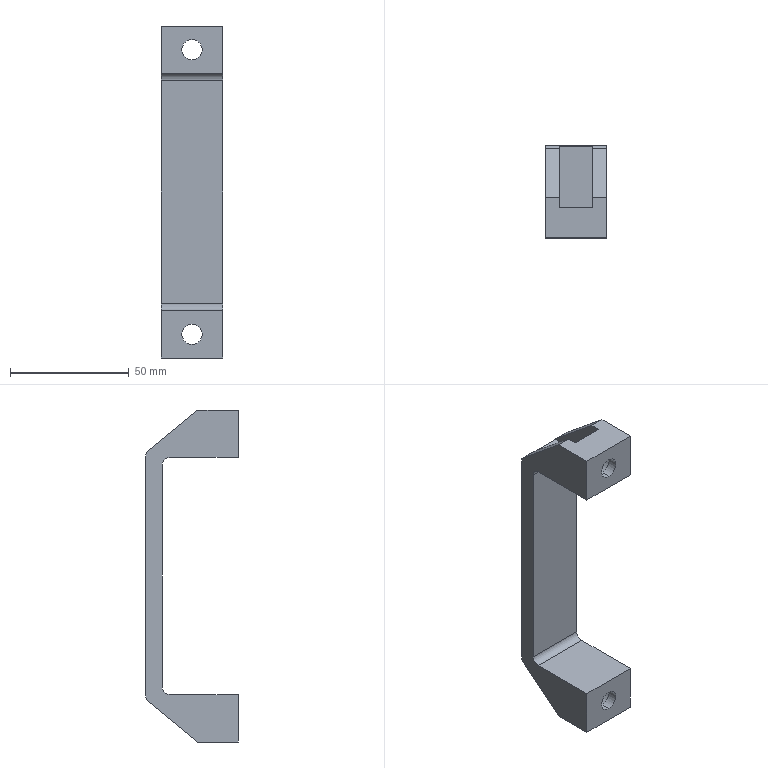Part | SolidWorks | features BaseBody 1 | 1 solid | 38 faces | box 26 x 39 x 140 mm | volume 37768 mm3 | plane 26 | cylinder 12 | commonest cylinder face diameters 6 x4 8.5 x4 14 x4
STEP:
#1=CARTESIAN_POINT('',(0.,-39.,-55.75));
#2=VERTEX_POINT('',#1);
#3=CARTESIAN_POINT('',(0.,-39.,-64.25));
#4=VERTEX_POINT('',#3);
#5=CARTESIAN_POINT('',(0.,-39.,-60.));
#6=DIRECTION('',(0.,-1.,0.));
#7=DIRECTION('',(0.,0.,1.));
#8=AXIS2_PLACEMENT_3D('',#5,#6,#7);
#9=CIRCLE('',#8,4.25);
#10=EDGE_CURVE('',#2,#4,#9,.T.);
#11=ORIENTED_EDGE('',*,*,#10,.T.);
#12=CARTESIAN_POINT('',(0.,-35.,-64.25));
#13=VERTEX_POINT('',#12);
#14=CARTESIAN_POINT('',(0.,-50.,-64.25));
#15=DIRECTION('',(0.,1.,0.));
#16=VECTOR('',#15,1000.);
#17=LINE('',#14,#16);
#18=EDGE_CURVE('',#4,#13,#17,.T.);
#19=ORIENTED_EDGE('',*,*,#18,.T.);
#20=CARTESIAN_POINT('',(0.,-35.,-55.75));
#21=VERTEX_POINT('',#20);
#22=CARTESIAN_POINT('',(0.,-35.,-60.));
#23=DIRECTION('',(0.,-1.,0.));
#24=DIRECTION('',(0.,0.,1.));
#25=AXIS2_PLACEMENT_3D('',#22,#23,#24);
#26=CIRCLE('',#25,4.25);
#27=EDGE_CURVE('',#21,#13,#26,.T.);
#28=ORIENTED_EDGE('',*,*,#27,.F.);
#29=CARTESIAN_POINT('',(0.,-50.,-55.75));
#30=DIRECTION('',(0.,1.,0.));
#31=VECTOR('',#30,1000.);
#32=LINE('',#29,#31);
#33=EDGE_CURVE('',#2,#21,#32,.T.);
#34=ORIENTED_EDGE('',*,*,#33,.F.);
#35=EDGE_LOOP('',(#11,#19,#28,#34));
#36=FACE_OUTER_BOUND('',#35,.T.);
#37=CARTESIAN_POINT('',(0.,-50.,-60.));
#38=DIRECTION('',(0.,1.,0.));
#39=DIRECTION('',(0.,0.,1.));
#40=AXIS2_PLACEMENT_3D('',#37,#38,#39);
#41=CYLINDRICAL_SURFACE('',#40,4.25);
#42=ADVANCED_FACE('',(#36),#41,.F.);
#43=CARTESIAN_POINT('',(0.,-35.,64.25));
#44=VERTEX_POINT('',#43);
#45=CARTESIAN_POINT('',(0.,-35.,55.75));
#46=VERTEX_POINT('',#45);
#47=CARTESIAN_POINT('',(0.,-35.,60.));
#48=DIRECTION('',(0.,-1.,0.));
#49=DIRECTION('',(0.,0.,-1.));
#50=AXIS2_PLACEMENT_3D('',#47,#48,#49);
#51=CIRCLE('',#50,4.25);
#52=EDGE_CURVE('',#44,#46,#51,.T.);
#53=ORIENTED_EDGE('',*,*,#52,.F.);
#54=CARTESIAN_POINT('',(0.,-39.,64.25));
#55=VERTEX_POINT('',#54);
#56=CARTESIAN_POINT('',(0.,50.,64.25));
#57=DIRECTION('',(0.,-1.,0.));
#58=VECTOR('',#57,1000.);
#59=LINE('',#56,#58);
#60=EDGE_CURVE('',#44,#55,#59,.T.);
#61=ORIENTED_EDGE('',*,*,#60,.T.);
#62=CARTESIAN_POINT('',(0.,-39.,55.75));
#63=VERTEX_POINT('',#62);
#64=CARTESIAN_POINT('',(0.,-39.,60.));
#65=DIRECTION('',(0.,-1.,0.));
#66=DIRECTION('',(0.,0.,-1.));
#67=AXIS2_PLACEMENT_3D('',#64,#65,#66);
#68=CIRCLE('',#67,4.25);
#69=EDGE_CURVE('',#55,#63,#68,.T.);
#70=ORIENTED_EDGE('',*,*,#69,.T.);
#71=CARTESIAN_POINT('',(0.,50.,55.75));
#72=DIRECTION('',(0.,-1.,0.));
#73=VECTOR('',#72,1000.);
#74=LINE('',#71,#73);
#75=EDGE_CURVE('',#46,#63,#74,.T.);
#76=ORIENTED_EDGE('',*,*,#75,.F.);
#77=EDGE_LOOP('',(#53,#61,#70,#76));
#78=FACE_OUTER_BOUND('',#77,.T.);
#79=CARTESIAN_POINT('',(0.,50.,60.));
#80=DIRECTION('',(0.,-1.,0.));
#81=DIRECTION('',(0.,0.,-1.));
#82=AXIS2_PLACEMENT_3D('',#79,#80,#81);
#83=CYLINDRICAL_SURFACE('',#82,4.25);
#84=ADVANCED_FACE('',(#78),#83,.F.);
#85=CARTESIAN_POINT('',(0.,-35.,-67.));
#86=VERTEX_POINT('',#85);
#87=CARTESIAN_POINT('',(0.,-35.,-53.));
#88=VERTEX_POINT('',#87);
#89=CARTESIAN_POINT('',(0.,-35.,-60.));
#90=DIRECTION('',(0.,1.,0.));
#91=DIRECTION('',(0.,0.,1.));
#92=AXIS2_PLACEMENT_3D('',#89,#90,#91);
#93=CIRCLE('',#92,7.);
#94=EDGE_CURVE('',#86,#88,#93,.T.);
#95=ORIENTED_EDGE('',*,*,#94,.F.);
#96=CARTESIAN_POINT('',(0.,-26.,-67.));
#97=VERTEX_POINT('',#96);
#98=CARTESIAN_POINT('',(0.,-50.,-67.));
#99=DIRECTION('',(0.,1.,0.));
#100=VECTOR('',#99,1000.);
#101=LINE('',#98,#100);
#102=EDGE_CURVE('',#86,#97,#101,.T.);
#103=ORIENTED_EDGE('',*,*,#102,.T.);
#104=CARTESIAN_POINT('',(-7.,-26.,-60.));
#105=VERTEX_POINT('',#104);
#106=CARTESIAN_POINT('',(0.,-26.,-60.));
#107=DIRECTION('',(0.,-1.,0.));
#108=DIRECTION('',(0.,0.,1.));
#109=AXIS2_PLACEMENT_3D('',#106,#107,#108);
#110=CIRCLE('',#109,7.);
#111=EDGE_CURVE('',#105,#97,#110,.T.);
#112=ORIENTED_EDGE('',*,*,#111,.F.);
#113=CARTESIAN_POINT('',(0.,-26.,-53.));
#114=VERTEX_POINT('',#113);
#115=CARTESIAN_POINT('',(0.,-26.,-60.));
#116=DIRECTION('',(0.,-1.,0.));
#117=DIRECTION('',(0.,0.,1.));
#118=AXIS2_PLACEMENT_3D('',#115,#116,#117);
#119=CIRCLE('',#118,7.);
#120=EDGE_CURVE('',#114,#105,#119,.T.);
#121=ORIENTED_EDGE('',*,*,#120,.F.);
#122=CARTESIAN_POINT('',(0.,-50.,-53.));
#123=DIRECTION('',(0.,1.,0.));
#124=VECTOR('',#123,1000.);
#125=LINE('',#122,#124);
#126=EDGE_CURVE('',#88,#114,#125,.T.);
#127=ORIENTED_EDGE('',*,*,#126,.F.);
#128=EDGE_LOOP('',(#95,#103,#112,#121,#127));
#129=FACE_OUTER_BOUND('',#128,.T.);
#130=CARTESIAN_POINT('',(0.,-50.,-60.));
#131=DIRECTION('',(0.,1.,0.));
#132=DIRECTION('',(0.,0.,1.));
#133=AXIS2_PLACEMENT_3D('',#130,#131,#132);
#134=CYLINDRICAL_SURFACE('',#133,7.);
#135=ADVANCED_FACE('',(#129),#134,.F.);
#136=CARTESIAN_POINT('',(0.,-26.,67.));
#137=VERTEX_POINT('',#136);
#138=CARTESIAN_POINT('',(-7.,-26.,60.));
#139=VERTEX_POINT('',#138);
#140=CARTESIAN_POINT('',(0.,-26.,60.));
#141=DIRECTION('',(0.,-1.,0.));
#142=DIRECTION('',(0.,0.,-1.));
#143=AXIS2_PLACEMENT_3D('',#140,#141,#142);
#144=CIRCLE('',#143,7.);
#145=EDGE_CURVE('',#137,#139,#144,.T.);
#146=ORIENTED_EDGE('',*,*,#145,.F.);
#147=CARTESIAN_POINT('',(0.,-35.,67.));
#148=VERTEX_POINT('',#147);
#149=CARTESIAN_POINT('',(0.,50.,67.));
#150=DIRECTION('',(0.,-1.,0.));
#151=VECTOR('',#150,1000.);
#152=LINE('',#149,#151);
#153=EDGE_CURVE('',#137,#148,#152,.T.);
#154=ORIENTED_EDGE('',*,*,#153,.T.);
#155=CARTESIAN_POINT('',(0.,-35.,53.));
#156=VERTEX_POINT('',#155);
#157=CARTESIAN_POINT('',(0.,-35.,60.));
#158=DIRECTION('',(0.,1.,0.));
#159=DIRECTION('',(0.,0.,-1.));
#160=AXIS2_PLACEMENT_3D('',#157,#158,#159);
#161=CIRCLE('',#160,7.);
#162=EDGE_CURVE('',#156,#148,#161,.T.);
#163=ORIENTED_EDGE('',*,*,#162,.F.);
#164=CARTESIAN_POINT('',(0.,-26.,53.));
#165=VERTEX_POINT('',#164);
#166=CARTESIAN_POINT('',(0.,50.,53.));
#167=DIRECTION('',(0.,-1.,0.));
#168=VECTOR('',#167,1000.);
#169=LINE('',#166,#168);
#170=EDGE_CURVE('',#165,#156,#169,.T.);
#171=ORIENTED_EDGE('',*,*,#170,.F.);
#172=CARTESIAN_POINT('',(0.,-26.,60.));
#173=DIRECTION('',(0.,-1.,0.));
#174=DIRECTION('',(0.,0.,-1.));
#175=AXIS2_PLACEMENT_3D('',#172,#173,#174);
#176=CIRCLE('',#175,7.);
#177=EDGE_CURVE('',#139,#165,#176,.T.);
#178=ORIENTED_EDGE('',*,*,#177,.F.);
#179=EDGE_LOOP('',(#146,#154,#163,#171,#178));
#180=FACE_OUTER_BOUND('',#179,.T.);
#181=CARTESIAN_POINT('',(0.,50.,60.));
#182=DIRECTION('',(0.,-1.,0.));
#183=DIRECTION('',(0.,0.,-1.));
#184=AXIS2_PLACEMENT_3D('',#181,#182,#183);
#185=CYLINDRICAL_SURFACE('',#184,7.);
#186=ADVANCED_FACE('',(#180),#185,.F.);
#187=CARTESIAN_POINT('',(13.,0.,50.578));
#188=VERTEX_POINT('',#187);
#189=CARTESIAN_POINT('',(-13.,0.,50.578));
#190=VERTEX_POINT('',#189);
#191=CARTESIAN_POINT('',(13.,0.,50.578));
#192=DIRECTION('',(-1.,0.,0.));
#193=VECTOR('',#192,1000.);
#194=LINE('',#191,#193);
#195=EDGE_CURVE('',#188,#190,#194,.T.);
#196=ORIENTED_EDGE('',*,*,#195,.F.);
#197=CARTESIAN_POINT('',(13.,0.,-50.578));
#198=VERTEX_POINT('',#197);
#199=CARTESIAN_POINT('',(13.,0.,-50.578));
#200=DIRECTION('',(0.,0.,1.));
#201=VECTOR('',#200,1000.);
#202=LINE('',#199,#201);
#203=EDGE_CURVE('',#198,#188,#202,.T.);
#204=ORIENTED_EDGE('',*,*,#203,.F.);
#205=CARTESIAN_POINT('',(-13.,0.,-50.578));
#206=VERTEX_POINT('',#205);
#207=CARTESIAN_POINT('',(13.,0.,-50.578));
#208=DIRECTION('',(1.,0.,0.));
#209=VECTOR('',#208,1000.);
#210=LINE('',#207,#209);
#211=EDGE_CURVE('',#206,#198,#210,.T.);
#212=ORIENTED_EDGE('',*,*,#211,.F.);
#213=CARTESIAN_POINT('',(-13.,0.,-50.578));
#214=DIRECTION('',(0.,0.,-1.));
#215=VECTOR('',#214,1000.);
#216=LINE('',#213,#215);
#217=EDGE_CURVE('',#190,#206,#216,.T.);
#218=ORIENTED_EDGE('',*,*,#217,.F.);
#219=EDGE_LOOP('',(#196,#204,#212,#218));
#220=FACE_OUTER_BOUND('',#219,.T.);
#221=CARTESIAN_POINT('',(13.,0.,-50.578));
#222=DIRECTION('',(0.,-1.,0.));
#223=DIRECTION('',(0.,0.,-1.));
#224=AXIS2_PLACEMENT_3D('',#221,#222,#223);
#225=PLANE('',#224);
#226=ADVANCED_FACE('',(#220),#225,.F.);
#227=ORIENTED_EDGE('',*,*,#217,.T.);
#228=CARTESIAN_POINT('',(-13.,-1.1,-52.9));
#229=VERTEX_POINT('',#228);
#230=CARTESIAN_POINT('',(-13.,-3.,-50.578));
#231=DIRECTION('',(1.,0.,0.));
#232=DIRECTION('',(0.,0.,-1.));
#233=AXIS2_PLACEMENT_3D('',#230,#231,#232);
#234=CIRCLE('',#233,3.);
#235=EDGE_CURVE('',#229,#206,#234,.T.);
#236=ORIENTED_EDGE('',*,*,#235,.F.);
#237=CARTESIAN_POINT('',(-13.,-22.,-70.));
#238=VERTEX_POINT('',#237);
#239=CARTESIAN_POINT('',(-13.,-22.,-70.));
#240=DIRECTION('',(0.,0.774,0.6332));
#241=VECTOR('',#240,1000.);
#242=LINE('',#239,#241);
#243=EDGE_CURVE('',#238,#229,#242,.T.);
#244=ORIENTED_EDGE('',*,*,#243,.F.);
#245=CARTESIAN_POINT('',(-13.,-39.,-70.));
#246=VERTEX_POINT('',#245);
#247=CARTESIAN_POINT('',(-13.,-10.,-70.));
#248=DIRECTION('',(0.,1.,0.));
#249=VECTOR('',#248,1000.);
#250=LINE('',#247,#249);
#251=EDGE_CURVE('',#246,#238,#250,.T.);
#252=ORIENTED_EDGE('',*,*,#251,.F.);
#253=CARTESIAN_POINT('',(-13.,-39.,-50.));
#254=VERTEX_POINT('',#253);
#255=CARTESIAN_POINT('',(-13.,-39.,47.));
#256=DIRECTION('',(0.,0.,-1.));
#257=VECTOR('',#256,1000.);
#258=LINE('',#255,#257);
#259=EDGE_CURVE('',#254,#246,#258,.T.);
#260=ORIENTED_EDGE('',*,*,#259,.F.);
#261=CARTESIAN_POINT('',(-13.,-10.,-50.));
#262=VERTEX_POINT('',#261);
#263=CARTESIAN_POINT('',(-13.,-10.,-50.));
#264=DIRECTION('',(0.,-1.,0.));
#265=VECTOR('',#264,1000.);
#266=LINE('',#263,#265);
#267=EDGE_CURVE('',#262,#254,#266,.T.);
#268=ORIENTED_EDGE('',*,*,#267,.F.);
#269=CARTESIAN_POINT('',(-13.,-7.,-47.));
#270=VERTEX_POINT('',#269);
#271=CARTESIAN_POINT('',(-13.,-10.,-47.));
#272=DIRECTION('',(-1.,0.,0.));
#273=DIRECTION('',(0.,0.,-1.));
#274=AXIS2_PLACEMENT_3D('',#271,#272,#273);
#275=CIRCLE('',#274,3.);
#276=EDGE_CURVE('',#270,#262,#275,.T.);
#277=ORIENTED_EDGE('',*,*,#276,.F.);
#278=CARTESIAN_POINT('',(-13.,-7.,47.));
#279=VERTEX_POINT('',#278);
#280=CARTESIAN_POINT('',(-13.,-7.,47.));
#281=DIRECTION('',(0.,0.,-1.));
#282=VECTOR('',#281,1000.);
#283=LINE('',#280,#282);
#284=EDGE_CURVE('',#279,#270,#283,.T.);
#285=ORIENTED_EDGE('',*,*,#284,.F.);
#286=CARTESIAN_POINT('',(-13.,-10.,50.));
#287=VERTEX_POINT('',#286);
#288=CARTESIAN_POINT('',(-13.,-10.,47.));
#289=DIRECTION('',(-1.,0.,0.));
#290=DIRECTION('',(0.,0.,-1.));
#291=AXIS2_PLACEMENT_3D('',#288,#289,#290);
#292=CIRCLE('',#291,3.);
#293=EDGE_CURVE('',#287,#279,#292,.T.);
#294=ORIENTED_EDGE('',*,*,#293,.F.);
#295=CARTESIAN_POINT('',(-13.,-39.,50.));
#296=VERTEX_POINT('',#295);
#297=CARTESIAN_POINT('',(-13.,-10.,50.));
#298=DIRECTION('',(0.,1.,0.));
#299=VECTOR('',#298,1000.);
#300=LINE('',#297,#299);
#301=EDGE_CURVE('',#296,#287,#300,.T.);
#302=ORIENTED_EDGE('',*,*,#301,.F.);
#303=CARTESIAN_POINT('',(-13.,-39.,70.));
#304=VERTEX_POINT('',#303);
#305=CARTESIAN_POINT('',(-13.,-39.,47.));
#306=DIRECTION('',(0.,0.,-1.));
#307=VECTOR('',#306,1000.);
#308=LINE('',#305,#307);
#309=EDGE_CURVE('',#304,#296,#308,.T.);
#310=ORIENTED_EDGE('',*,*,#309,.F.);
#311=CARTESIAN_POINT('',(-13.,-22.,70.));
#312=VERTEX_POINT('',#311);
#313=CARTESIAN_POINT('',(-13.,-10.,70.));
#314=DIRECTION('',(0.,-1.,0.));
#315=VECTOR('',#314,1000.);
#316=LINE('',#313,#315);
#317=EDGE_CURVE('',#312,#304,#316,.T.);
#318=ORIENTED_EDGE('',*,*,#317,.F.);
#319=CARTESIAN_POINT('',(-13.,-1.1,52.9));
#320=VERTEX_POINT('',#319);
#321=CARTESIAN_POINT('',(-13.,-1.1,52.9));
#322=DIRECTION('',(0.,-0.774,0.6332));
#323=VECTOR('',#322,1000.);
#324=LINE('',#321,#323);
#325=EDGE_CURVE('',#320,#312,#324,.T.);
#326=ORIENTED_EDGE('',*,*,#325,.F.);
#327=CARTESIAN_POINT('',(-13.,-3.,50.578));
#328=DIRECTION('',(1.,0.,0.));
#329=DIRECTION('',(0.,0.,-1.));
#330=AXIS2_PLACEMENT_3D('',#327,#328,#329);
#331=CIRCLE('',#330,3.);
#332=EDGE_CURVE('',#190,#320,#331,.T.);
#333=ORIENTED_EDGE('',*,*,#332,.F.);
#334=EDGE_LOOP('',(#227,#236,#244,#252,#260,#268,#277,#285,#294,#302,#310,#318,#326,#333));
#335=FACE_OUTER_BOUND('',#334,.T.);
#336=CARTESIAN_POINT('',(-13.,-10.,47.));
#337=DIRECTION('',(1.,0.,0.));
#338=DIRECTION('',(0.,0.,-1.));
#339=AXIS2_PLACEMENT_3D('',#336,#337,#338);
#340=PLANE('',#339);
#341=ADVANCED_FACE('',(#335),#340,.F.);
#342=ORIENTED_EDGE('',*,*,#195,.T.);
#343=ORIENTED_EDGE('',*,*,#332,.T.);
#344=CARTESIAN_POINT('',(-7.,-1.1,52.9));
#345=VERTEX_POINT('',#344);
#346=CARTESIAN_POINT('',(13.,-1.1,52.9));
#347=DIRECTION('',(1.,0.,0.));
#348=VECTOR('',#347,1000.);
#349=LINE('',#346,#348);
#350=EDGE_CURVE('',#320,#345,#349,.T.);
#351=ORIENTED_EDGE('',*,*,#350,.T.);
#352=CARTESIAN_POINT('',(-7.,-0.3582,52.));
#353=VERTEX_POINT('',#352);
#354=CARTESIAN_POINT('',(-7.,-3.,50.578));
#355=DIRECTION('',(1.,0.,0.));
#356=DIRECTION('',(0.,0.,-1.));
#357=AXIS2_PLACEMENT_3D('',#354,#355,#356);
#358=CIRCLE('',#357,3.);
#359=EDGE_CURVE('',#353,#345,#358,.T.);
#360=ORIENTED_EDGE('',*,*,#359,.F.);
#361=CARTESIAN_POINT('',(7.,-0.3582,52.));
#362=VERTEX_POINT('',#361);
#363=CARTESIAN_POINT('',(13.,-0.3582,52.));
#364=DIRECTION('',(1.,0.,0.));
#365=VECTOR('',#364,1000.);
#366=LINE('',#363,#365);
#367=EDGE_CURVE('',#353,#362,#366,.T.);
#368=ORIENTED_EDGE('',*,*,#367,.T.);
#369=CARTESIAN_POINT('',(7.,-1.1,52.9));
#370=VERTEX_POINT('',#369);
#371=CARTESIAN_POINT('',(7.,-3.,50.578));
#372=DIRECTION('',(1.,0.,0.));
#373=DIRECTION('',(0.,0.,-1.));
#374=AXIS2_PLACEMENT_3D('',#371,#372,#373);
#375=CIRCLE('',#374,3.);
#376=EDGE_CURVE('',#362,#370,#375,.T.);
#377=ORIENTED_EDGE('',*,*,#376,.T.);
#378=CARTESIAN_POINT('',(13.,-1.1,52.9));
#379=VERTEX_POINT('',#378);
#380=CARTESIAN_POINT('',(13.,-1.1,52.9));
#381=DIRECTION('',(1.,0.,0.));
#382=VECTOR('',#381,1000.);
#383=LINE('',#380,#382);
#384=EDGE_CURVE('',#370,#379,#383,.T.);
#385=ORIENTED_EDGE('',*,*,#384,.T.);
#386=CARTESIAN_POINT('',(13.,-3.,50.578));
#387=DIRECTION('',(-1.,0.,0.));
#388=DIRECTION('',(0.,0.,-1.));
#389=AXIS2_PLACEMENT_3D('',#386,#387,#388);
#390=CIRCLE('',#389,3.);
#391=EDGE_CURVE('',#379,#188,#390,.T.);
#392=ORIENTED_EDGE('',*,*,#391,.T.);
#393=EDGE_LOOP('',(#342,#343,#351,#360,#368,#377,#385,#392));
#394=FACE_OUTER_BOUND('',#393,.T.);
#395=CARTESIAN_POINT('',(13.,-3.,50.578));
#396=DIRECTION('',(1.,0.,0.));
#397=DIRECTION('',(0.,0.,-1.));
#398=AXIS2_PLACEMENT_3D('',#395,#396,#397);
#399=CYLINDRICAL_SURFACE('',#398,3.);
#400=ADVANCED_FACE('',(#394),#399,.T.);
#401=CARTESIAN_POINT('',(13.,-22.,-70.));
#402=VERTEX_POINT('',#401);
#403=CARTESIAN_POINT('',(13.,-1.1,-52.9));
#404=VERTEX_POINT('',#403);
#405=CARTESIAN_POINT('',(13.,-22.,-70.));
#406=DIRECTION('',(0.,0.774,0.6332));
#407=VECTOR('',#406,1000.);
#408=LINE('',#405,#407);
#409=EDGE_CURVE('',#402,#404,#408,.T.);
#410=ORIENTED_EDGE('',*,*,#409,.T.);
#411=CARTESIAN_POINT('',(13.,-3.,-50.578));
#412=DIRECTION('',(1.,0.,0.));
#413=DIRECTION('',(0.,0.,-1.));
#414=AXIS2_PLACEMENT_3D('',#411,#412,#413);
#415=CIRCLE('',#414,3.);
#416=EDGE_CURVE('',#404,#198,#415,.T.);
#417=ORIENTED_EDGE('',*,*,#416,.T.);
#418=ORIENTED_EDGE('',*,*,#203,.T.);
#419=ORIENTED_EDGE('',*,*,#391,.F.);
#420=CARTESIAN_POINT('',(13.,-22.,70.));
#421=VERTEX_POINT('',#420);
#422=CARTESIAN_POINT('',(13.,-1.1,52.9));
#423=DIRECTION('',(0.,-0.774,0.6332));
#424=VECTOR('',#423,1000.);
#425=LINE('',#422,#424);
#426=EDGE_CURVE('',#379,#421,#425,.T.);
#427=ORIENTED_EDGE('',*,*,#426,.T.);
#428=CARTESIAN_POINT('',(13.,-39.,70.));
#429=VERTEX_POINT('',#428);
#430=CARTESIAN_POINT('',(13.,-10.,70.));
#431=DIRECTION('',(0.,-1.,0.));
#432=VECTOR('',#431,1000.);
#433=LINE('',#430,#432);
#434=EDGE_CURVE('',#421,#429,#433,.T.);
#435=ORIENTED_EDGE('',*,*,#434,.T.);
#436=CARTESIAN_POINT('',(13.,-39.,50.));
#437=VERTEX_POINT('',#436);
#438=CARTESIAN_POINT('',(13.,-39.,47.));
#439=DIRECTION('',(0.,0.,-1.));
#440=VECTOR('',#439,1000.);
#441=LINE('',#438,#440);
#442=EDGE_CURVE('',#429,#437,#441,.T.);
#443=ORIENTED_EDGE('',*,*,#442,.T.);
#444=CARTESIAN_POINT('',(13.,-10.,50.));
#445=VERTEX_POINT('',#444);
#446=CARTESIAN_POINT('',(13.,-10.,50.));
#447=DIRECTION('',(0.,1.,0.));
#448=VECTOR('',#447,1000.);
#449=LINE('',#446,#448);
#450=EDGE_CURVE('',#437,#445,#449,.T.);
#451=ORIENTED_EDGE('',*,*,#450,.T.);
#452=CARTESIAN_POINT('',(13.,-7.,47.));
#453=VERTEX_POINT('',#452);
#454=CARTESIAN_POINT('',(13.,-10.,47.));
#455=DIRECTION('',(-1.,0.,0.));
#456=DIRECTION('',(0.,0.,-1.));
#457=AXIS2_PLACEMENT_3D('',#454,#455,#456);
#458=CIRCLE('',#457,3.);
#459=EDGE_CURVE('',#445,#453,#458,.T.);
#460=ORIENTED_EDGE('',*,*,#459,.T.);
#461=CARTESIAN_POINT('',(13.,-7.,-47.));
#462=VERTEX_POINT('',#461);
#463=CARTESIAN_POINT('',(13.,-7.,47.));
#464=DIRECTION('',(0.,0.,-1.));
#465=VECTOR('',#464,1000.);
#466=LINE('',#463,#465);
#467=EDGE_CURVE('',#453,#462,#466,.T.);
#468=ORIENTED_EDGE('',*,*,#467,.T.);
#469=CARTESIAN_POINT('',(13.,-10.,-50.));
#470=VERTEX_POINT('',#469);
#471=CARTESIAN_POINT('',(13.,-10.,-47.));
#472=DIRECTION('',(-1.,0.,0.));
#473=DIRECTION('',(0.,0.,-1.));
#474=AXIS2_PLACEMENT_3D('',#471,#472,#473);
#475=CIRCLE('',#474,3.);
#476=EDGE_CURVE('',#462,#470,#475,.T.);
#477=ORIENTED_EDGE('',*,*,#476,.T.);
#478=CARTESIAN_POINT('',(13.,-39.,-50.));
#479=VERTEX_POINT('',#478);
#480=CARTESIAN_POINT('',(13.,-10.,-50.));
#481=DIRECTION('',(0.,-1.,0.));
#482=VECTOR('',#481,1000.);
#483=LINE('',#480,#482);
#484=EDGE_CURVE('',#470,#479,#483,.T.);
#485=ORIENTED_EDGE('',*,*,#484,.T.);
#486=CARTESIAN_POINT('',(13.,-39.,-70.));
#487=VERTEX_POINT('',#486);
#488=CARTESIAN_POINT('',(13.,-39.,47.));
#489=DIRECTION('',(0.,0.,-1.));
#490=VECTOR('',#489,1000.);
#491=LINE('',#488,#490);
#492=EDGE_CURVE('',#479,#487,#491,.T.);
#493=ORIENTED_EDGE('',*,*,#492,.T.);
#494=CARTESIAN_POINT('',(13.,-10.,-70.));
#495=DIRECTION('',(0.,1.,0.));
#496=VECTOR('',#495,1000.);
#497=LINE('',#494,#496);
#498=EDGE_CURVE('',#487,#402,#497,.T.);
#499=ORIENTED_EDGE('',*,*,#498,.T.);
#500=EDGE_LOOP('',(#410,#417,#418,#419,#427,#435,#443,#451,#460,#468,#477,#485,#493,#499));
#501=FACE_OUTER_BOUND('',#500,.T.);
#502=CARTESIAN_POINT('',(13.,-10.,47.));
#503=DIRECTION('',(1.,0.,0.));
#504=DIRECTION('',(0.,0.,-1.));
#505=AXIS2_PLACEMENT_3D('',#502,#503,#504);
#506=PLANE('',#505);
#507=ADVANCED_FACE('',(#501),#506,.T.);
#508=CARTESIAN_POINT('',(-7.,-1.1,-52.9));
#509=VERTEX_POINT('',#508);
#510=CARTESIAN_POINT('',(13.,-1.1,-52.9));
#511=DIRECTION('',(-1.,0.,0.));
#512=VECTOR('',#511,1000.);
#513=LINE('',#510,#512);
#514=EDGE_CURVE('',#509,#229,#513,.T.);
#515=ORIENTED_EDGE('',*,*,#514,.T.);
#516=ORIENTED_EDGE('',*,*,#235,.T.);
#517=ORIENTED_EDGE('',*,*,#211,.T.);
#518=ORIENTED_EDGE('',*,*,#416,.F.);
#519=CARTESIAN_POINT('',(7.,-1.1,-52.9));
#520=VERTEX_POINT('',#519);
#521=CARTESIAN_POINT('',(13.,-1.1,-52.9));
#522=DIRECTION('',(-1.,0.,0.));
#523=VECTOR('',#522,1000.);
#524=LINE('',#521,#523);
#525=EDGE_CURVE('',#404,#520,#524,.T.);
#526=ORIENTED_EDGE('',*,*,#525,.T.);
#527=CARTESIAN_POINT('',(7.,-0.3582,-52.));
#528=VERTEX_POINT('',#527);
#529=CARTESIAN_POINT('',(7.,-3.,-50.578));
#530=DIRECTION('',(1.,0.,0.));
#531=DIRECTION('',(0.,0.,-1.));
#532=AXIS2_PLACEMENT_3D('',#529,#530,#531);
#533=CIRCLE('',#532,3.);
#534=EDGE_CURVE('',#520,#528,#533,.T.);
#535=ORIENTED_EDGE('',*,*,#534,.T.);
#536=CARTESIAN_POINT('',(-7.,-0.3582,-52.));
#537=VERTEX_POINT('',#536);
#538=CARTESIAN_POINT('',(13.,-0.3582,-52.));
#539=DIRECTION('',(-1.,0.,0.));
#540=VECTOR('',#539,1000.);
#541=LINE('',#538,#540);
#542=EDGE_CURVE('',#528,#537,#541,.T.);
#543=ORIENTED_EDGE('',*,*,#542,.T.);
#544=CARTESIAN_POINT('',(-7.,-3.,-50.578));
#545=DIRECTION('',(1.,0.,0.));
#546=DIRECTION('',(0.,0.,-1.));
#547=AXIS2_PLACEMENT_3D('',#544,#545,#546);
#548=CIRCLE('',#547,3.);
#549=EDGE_CURVE('',#509,#537,#548,.T.);
#550=ORIENTED_EDGE('',*,*,#549,.F.);
#551=EDGE_LOOP('',(#515,#516,#517,#518,#526,#535,#543,#550));
#552=FACE_OUTER_BOUND('',#551,.T.);
#553=CARTESIAN_POINT('',(13.,-3.,-50.578));
#554=DIRECTION('',(1.,0.,0.));
#555=DIRECTION('',(0.,0.,-1.));
#556=AXIS2_PLACEMENT_3D('',#553,#554,#555);
#557=CYLINDRICAL_SURFACE('',#556,3.);
#558=ADVANCED_FACE('',(#552),#557,.T.);
#559=ORIENTED_EDGE('',*,*,#243,.T.);
#560=ORIENTED_EDGE('',*,*,#514,.F.);
#561=CARTESIAN_POINT('',(-7.,-22.,-70.));
#562=VERTEX_POINT('',#561);
#563=CARTESIAN_POINT('',(-7.,-22.,-70.));
#564=DIRECTION('',(0.,0.774,0.6332));
#565=VECTOR('',#564,1000.);
#566=LINE('',#563,#565);
#567=EDGE_CURVE('',#562,#509,#566,.T.);
#568=ORIENTED_EDGE('',*,*,#567,.F.);
#569=CARTESIAN_POINT('',(13.,-22.,-70.));
#570=DIRECTION('',(1.,0.,0.));
#571=VECTOR('',#570,1000.);
#572=LINE('',#569,#571);
#573=EDGE_CURVE('',#238,#562,#572,.T.);
#574=ORIENTED_EDGE('',*,*,#573,.F.);
#575=EDGE_LOOP('',(#559,#560,#568,#574));
#576=FACE_OUTER_BOUND('',#575,.T.);
#577=CARTESIAN_POINT('',(13.,-22.,-70.));
#578=DIRECTION('',(0.,-0.6332,0.774));
#579=DIRECTION('',(0.,-0.774,-0.6332));
#580=AXIS2_PLACEMENT_3D('',#577,#578,#579);
#581=PLANE('',#580);
#582=ADVANCED_FACE('',(#576),#581,.F.);
#583=CARTESIAN_POINT('',(7.,-22.,-70.));
#584=VERTEX_POINT('',#583);
#585=CARTESIAN_POINT('',(13.,-22.,-70.));
#586=DIRECTION('',(-1.,0.,0.));
#587=VECTOR('',#586,1000.);
#588=LINE('',#585,#587);
#589=EDGE_CURVE('',#402,#584,#588,.T.);
#590=ORIENTED_EDGE('',*,*,#589,.F.);
#591=ORIENTED_EDGE('',*,*,#498,.F.);
#592=CARTESIAN_POINT('',(13.,-39.,-70.));
#593=DIRECTION('',(1.,0.,0.));
#594=VECTOR('',#593,1000.);
#595=LINE('',#592,#594);
#596=EDGE_CURVE('',#246,#487,#595,.T.);
#597=ORIENTED_EDGE('',*,*,#596,.F.);
#598=ORIENTED_EDGE('',*,*,#251,.T.);
#599=ORIENTED_EDGE('',*,*,#573,.T.);
#600=CARTESIAN_POINT('',(-7.,-26.,-70.));
#601=VERTEX_POINT('',#600);
#602=CARTESIAN_POINT('',(-7.,-39.,-70.));
#603=DIRECTION('',(0.,1.,0.));
#604=VECTOR('',#603,1000.);
#605=LINE('',#602,#604);
#606=EDGE_CURVE('',#601,#562,#605,.T.);
#607=ORIENTED_EDGE('',*,*,#606,.F.);
#608=CARTESIAN_POINT('',(7.,-26.,-70.));
#609=VERTEX_POINT('',#608);
#610=CARTESIAN_POINT('',(13.,-26.,-70.));
#611=DIRECTION('',(-1.,0.,0.));
#612=VECTOR('',#611,1000.);
#613=LINE('',#610,#612);
#614=EDGE_CURVE('',#609,#601,#613,.T.);
#615=ORIENTED_EDGE('',*,*,#614,.F.);
#616=CARTESIAN_POINT('',(7.,-39.,-70.));
#617=DIRECTION('',(0.,-1.,0.));
#618=VECTOR('',#617,1000.);
#619=LINE('',#616,#618);
#620=EDGE_CURVE('',#584,#609,#619,.T.);
#621=ORIENTED_EDGE('',*,*,#620,.F.);
#622=EDGE_LOOP('',(#590,#591,#597,#598,#599,#607,#615,#621));
#623=FACE_OUTER_BOUND('',#622,.T.);
#624=CARTESIAN_POINT('',(13.,-39.,-70.));
#625=DIRECTION('',(0.,0.,1.));
#626=DIRECTION('',(1.,0.,0.));
#627=AXIS2_PLACEMENT_3D('',#624,#625,#626);
#628=PLANE('',#627);
#629=ADVANCED_FACE('',(#623),#628,.F.);
#630=ORIENTED_EDGE('',*,*,#10,.F.);
#631=CARTESIAN_POINT('',(0.,-39.,-60.));
#632=DIRECTION('',(0.,-1.,0.));
#633=DIRECTION('',(0.,0.,1.));
#634=AXIS2_PLACEMENT_3D('',#631,#632,#633);
#635=CIRCLE('',#634,4.25);
#636=EDGE_CURVE('',#4,#2,#635,.T.);
#637=ORIENTED_EDGE('',*,*,#636,.F.);
#638=EDGE_LOOP('',(#630,#637));
#639=FACE_BOUND('',#638,.T.);
#640=ORIENTED_EDGE('',*,*,#492,.F.);
#641=CARTESIAN_POINT('',(13.,-39.,-50.));
#642=DIRECTION('',(1.,0.,0.));
#643=VECTOR('',#642,1000.);
#644=LINE('',#641,#643);
#645=EDGE_CURVE('',#254,#479,#644,.T.);
#646=ORIENTED_EDGE('',*,*,#645,.F.);
#647=ORIENTED_EDGE('',*,*,#259,.T.);
#648=ORIENTED_EDGE('',*,*,#596,.T.);
#649=EDGE_LOOP('',(#640,#646,#647,#648));
#650=FACE_OUTER_BOUND('',#649,.T.);
#651=CARTESIAN_POINT('',(13.,-39.,-50.));
#652=DIRECTION('',(0.,1.,0.));
#653=DIRECTION('',(0.,0.,1.));
#654=AXIS2_PLACEMENT_3D('',#651,#652,#653);
#655=PLANE('',#654);
#656=ADVANCED_FACE('',(#639,#650),#655,.F.);
#657=ORIENTED_EDGE('',*,*,#484,.F.);
#658=CARTESIAN_POINT('',(13.,-10.,-50.));
#659=DIRECTION('',(1.,0.,0.));
#660=VECTOR('',#659,1000.);
#661=LINE('',#658,#660);
#662=EDGE_CURVE('',#262,#470,#661,.T.);
#663=ORIENTED_EDGE('',*,*,#662,.F.);
#664=ORIENTED_EDGE('',*,*,#267,.T.);
#665=ORIENTED_EDGE('',*,*,#645,.T.);
#666=EDGE_LOOP('',(#657,#663,#664,#665));
#667=FACE_OUTER_BOUND('',#666,.T.);
#668=CARTESIAN_POINT('',(13.,-10.,-50.));
#669=DIRECTION('',(0.,0.,-1.));
#670=DIRECTION('',(-1.,0.,0.));
#671=AXIS2_PLACEMENT_3D('',#668,#669,#670);
#672=PLANE('',#671);
#673=ADVANCED_FACE('',(#667),#672,.F.);
#674=ORIENTED_EDGE('',*,*,#476,.F.);
#675=CARTESIAN_POINT('',(13.,-7.,-47.));
#676=DIRECTION('',(1.,0.,0.));
#677=VECTOR('',#676,1000.);
#678=LINE('',#675,#677);
#679=EDGE_CURVE('',#270,#462,#678,.T.);
#680=ORIENTED_EDGE('',*,*,#679,.F.);
#681=ORIENTED_EDGE('',*,*,#276,.T.);
#682=ORIENTED_EDGE('',*,*,#662,.T.);
#683=EDGE_LOOP('',(#674,#680,#681,#682));
#684=FACE_OUTER_BOUND('',#683,.T.);
#685=CARTESIAN_POINT('',(13.,-10.,-47.));
#686=DIRECTION('',(1.,0.,0.));
#687=DIRECTION('',(0.,0.,-1.));
#688=AXIS2_PLACEMENT_3D('',#685,#686,#687);
#689=CYLINDRICAL_SURFACE('',#688,3.);
#690=ADVANCED_FACE('',(#684),#689,.F.);
#691=ORIENTED_EDGE('',*,*,#467,.F.);
#692=CARTESIAN_POINT('',(13.,-7.,47.));
#693=DIRECTION('',(1.,0.,0.));
#694=VECTOR('',#693,1000.);
#695=LINE('',#692,#694);
#696=EDGE_CURVE('',#279,#453,#695,.T.);
#697=ORIENTED_EDGE('',*,*,#696,.F.);
#698=ORIENTED_EDGE('',*,*,#284,.T.);
#699=ORIENTED_EDGE('',*,*,#679,.T.);
#700=EDGE_LOOP('',(#691,#697,#698,#699));
#701=FACE_OUTER_BOUND('',#700,.T.);
#702=CARTESIAN_POINT('',(13.,-7.,47.));
#703=DIRECTION('',(0.,1.,0.));
#704=DIRECTION('',(0.,0.,1.));
#705=AXIS2_PLACEMENT_3D('',#702,#703,#704);
#706=PLANE('',#705);
#707=ADVANCED_FACE('',(#701),#706,.F.);
#708=ORIENTED_EDGE('',*,*,#459,.F.);
#709=CARTESIAN_POINT('',(13.,-10.,50.));
#710=DIRECTION('',(1.,0.,0.));
#711=VECTOR('',#710,1000.);
#712=LINE('',#709,#711);
#713=EDGE_CURVE('',#287,#445,#712,.T.);
#714=ORIENTED_EDGE('',*,*,#713,.F.);
#715=ORIENTED_EDGE('',*,*,#293,.T.);
#716=ORIENTED_EDGE('',*,*,#696,.T.);
#717=EDGE_LOOP('',(#708,#714,#715,#716));
#718=FACE_OUTER_BOUND('',#717,.T.);
#719=CARTESIAN_POINT('',(13.,-10.,47.));
#720=DIRECTION('',(1.,0.,0.));
#721=DIRECTION('',(0.,0.,-1.));
#722=AXIS2_PLACEMENT_3D('',#719,#720,#721);
#723=CYLINDRICAL_SURFACE('',#722,3.);
#724=ADVANCED_FACE('',(#718),#723,.F.);
#725=ORIENTED_EDGE('',*,*,#450,.F.);
#726=CARTESIAN_POINT('',(13.,-39.,50.));
#727=DIRECTION('',(1.,0.,0.));
#728=VECTOR('',#727,1000.);
#729=LINE('',#726,#728);
#730=EDGE_CURVE('',#296,#437,#729,.T.);
#731=ORIENTED_EDGE('',*,*,#730,.F.);
#732=ORIENTED_EDGE('',*,*,#301,.T.);
#733=ORIENTED_EDGE('',*,*,#713,.T.);
#734=EDGE_LOOP('',(#725,#731,#732,#733));
#735=FACE_OUTER_BOUND('',#734,.T.);
#736=CARTESIAN_POINT('',(13.,-39.,50.));
#737=DIRECTION('',(0.,0.,1.));
#738=DIRECTION('',(1.,0.,0.));
#739=AXIS2_PLACEMENT_3D('',#736,#737,#738);
#740=PLANE('',#739);
#741=ADVANCED_FACE('',(#735),#740,.F.);
#742=CARTESIAN_POINT('',(0.,-39.,60.));
#743=DIRECTION('',(0.,-1.,0.));
#744=DIRECTION('',(0.,0.,-1.));
#745=AXIS2_PLACEMENT_3D('',#742,#743,#744);
#746=CIRCLE('',#745,4.25);
#747=EDGE_CURVE('',#63,#55,#746,.T.);
#748=ORIENTED_EDGE('',*,*,#747,.F.);
#749=ORIENTED_EDGE('',*,*,#69,.F.);
#750=EDGE_LOOP('',(#748,#749));
#751=FACE_BOUND('',#750,.T.);
#752=ORIENTED_EDGE('',*,*,#442,.F.);
#753=CARTESIAN_POINT('',(13.,-39.,70.));
#754=DIRECTION('',(1.,0.,0.));
#755=VECTOR('',#754,1000.);
#756=LINE('',#753,#755);
#757=EDGE_CURVE('',#304,#429,#756,.T.);
#758=ORIENTED_EDGE('',*,*,#757,.F.);
#759=ORIENTED_EDGE('',*,*,#309,.T.);
#760=ORIENTED_EDGE('',*,*,#730,.T.);
#761=EDGE_LOOP('',(#752,#758,#759,#760));
#762=FACE_OUTER_BOUND('',#761,.T.);
#763=CARTESIAN_POINT('',(13.,-39.,70.));
#764=DIRECTION('',(0.,1.,0.));
#765=DIRECTION('',(0.,0.,1.));
#766=AXIS2_PLACEMENT_3D('',#763,#764,#765);
#767=PLANE('',#766);
#768=ADVANCED_FACE('',(#751,#762),#767,.F.);
#769=CARTESIAN_POINT('',(-7.,-26.,70.));
#770=VERTEX_POINT('',#769);
#771=CARTESIAN_POINT('',(7.,-26.,70.));
#772=VERTEX_POINT('',#771);
#773=CARTESIAN_POINT('',(13.,-26.,70.));
#774=DIRECTION('',(1.,0.,0.));
#775=VECTOR('',#774,1000.);
#776=LINE('',#773,#775);
#777=EDGE_CURVE('',#770,#772,#776,.T.);
#778=ORIENTED_EDGE('',*,*,#777,.F.);
#779=CARTESIAN_POINT('',(-7.,-22.,70.));
#780=VERTEX_POINT('',#779);
#781=CARTESIAN_POINT('',(-7.,-22.,70.));
#782=DIRECTION('',(0.,-1.,0.));
#783=VECTOR('',#782,1000.);
#784=LINE('',#781,#783);
#785=EDGE_CURVE('',#780,#770,#784,.T.);
#786=ORIENTED_EDGE('',*,*,#785,.F.);
#787=CARTESIAN_POINT('',(13.,-22.,70.));
#788=DIRECTION('',(1.,0.,0.));
#789=VECTOR('',#788,1000.);
#790=LINE('',#787,#789);
#791=EDGE_CURVE('',#312,#780,#790,.T.);
#792=ORIENTED_EDGE('',*,*,#791,.F.);
#793=ORIENTED_EDGE('',*,*,#317,.T.);
#794=ORIENTED_EDGE('',*,*,#757,.T.);
#795=ORIENTED_EDGE('',*,*,#434,.F.);
#796=CARTESIAN_POINT('',(7.,-22.,70.));
#797=VERTEX_POINT('',#796);
#798=CARTESIAN_POINT('',(13.,-22.,70.));
#799=DIRECTION('',(1.,0.,0.));
#800=VECTOR('',#799,1000.);
#801=LINE('',#798,#800);
#802=EDGE_CURVE('',#797,#421,#801,.T.);
#803=ORIENTED_EDGE('',*,*,#802,.F.);
#804=CARTESIAN_POINT('',(7.,-22.,70.));
#805=DIRECTION('',(0.,1.,0.));
#806=VECTOR('',#805,1000.);
#807=LINE('',#804,#806);
#808=EDGE_CURVE('',#772,#797,#807,.T.);
#809=ORIENTED_EDGE('',*,*,#808,.F.);
#810=EDGE_LOOP('',(#778,#786,#792,#793,#794,#795,#803,#809));
#811=FACE_OUTER_BOUND('',#810,.T.);
#812=CARTESIAN_POINT('',(13.,-22.,70.));
#813=DIRECTION('',(0.,0.,-1.));
#814=DIRECTION('',(-1.,0.,0.));
#815=AXIS2_PLACEMENT_3D('',#812,#813,#814);
#816=PLANE('',#815);
#817=ADVANCED_FACE('',(#811),#816,.F.);
#818=ORIENTED_EDGE('',*,*,#325,.T.);
#819=ORIENTED_EDGE('',*,*,#791,.T.);
#820=CARTESIAN_POINT('',(-7.,-1.1,52.9));
#821=DIRECTION('',(0.,-0.774,0.6332));
#822=VECTOR('',#821,1000.);
#823=LINE('',#820,#822);
#824=EDGE_CURVE('',#345,#780,#823,.T.);
#825=ORIENTED_EDGE('',*,*,#824,.F.);
#826=ORIENTED_EDGE('',*,*,#350,.F.);
#827=EDGE_LOOP('',(#818,#819,#825,#826));
#828=FACE_OUTER_BOUND('',#827,.T.);
#829=CARTESIAN_POINT('',(13.,-1.1,52.9));
#830=DIRECTION('',(0.,-0.6332,-0.774));
#831=DIRECTION('',(0.,0.774,-0.6332));
#832=AXIS2_PLACEMENT_3D('',#829,#830,#831);
#833=PLANE('',#832);
#834=ADVANCED_FACE('',(#828),#833,.F.);
#835=ORIENTED_EDGE('',*,*,#802,.T.);
#836=ORIENTED_EDGE('',*,*,#426,.F.);
#837=ORIENTED_EDGE('',*,*,#384,.F.);
#838=CARTESIAN_POINT('',(7.,-1.1,52.9));
#839=DIRECTION('',(0.,0.774,-0.6332));
#840=VECTOR('',#839,1000.);
#841=LINE('',#838,#840);
#842=EDGE_CURVE('',#797,#370,#841,.T.);
#843=ORIENTED_EDGE('',*,*,#842,.F.);
#844=EDGE_LOOP('',(#835,#836,#837,#843));
#845=FACE_OUTER_BOUND('',#844,.T.);
#846=CARTESIAN_POINT('',(13.,-1.1,52.9));
#847=DIRECTION('',(0.,-0.6332,-0.774));
#848=DIRECTION('',(0.,0.774,-0.6332));
#849=AXIS2_PLACEMENT_3D('',#846,#847,#848);
#850=PLANE('',#849);
#851=ADVANCED_FACE('',(#845),#850,.F.);
#852=ORIENTED_EDGE('',*,*,#367,.F.);
#853=CARTESIAN_POINT('',(-7.,-26.,52.));
#854=VERTEX_POINT('',#853);
#855=CARTESIAN_POINT('',(-7.,-26.,52.));
#856=DIRECTION('',(0.,-1.,0.));
#857=VECTOR('',#856,1000.);
#858=LINE('',#855,#857);
#859=EDGE_CURVE('',#353,#854,#858,.T.);
#860=ORIENTED_EDGE('',*,*,#859,.T.);
#861=CARTESIAN_POINT('',(7.,-26.,52.));
#862=VERTEX_POINT('',#861);
#863=CARTESIAN_POINT('',(7.,-26.,52.));
#864=DIRECTION('',(1.,0.,0.));
#865=VECTOR('',#864,1000.);
#866=LINE('',#863,#865);
#867=EDGE_CURVE('',#854,#862,#866,.T.);
#868=ORIENTED_EDGE('',*,*,#867,.T.);
#869=CARTESIAN_POINT('',(7.,-26.,52.));
#870=DIRECTION('',(0.,1.,0.));
#871=VECTOR('',#870,1000.);
#872=LINE('',#869,#871);
#873=EDGE_CURVE('',#862,#362,#872,.T.);
#874=ORIENTED_EDGE('',*,*,#873,.T.);
#875=EDGE_LOOP('',(#852,#860,#868,#874));
#876=FACE_OUTER_BOUND('',#875,.T.);
#877=CARTESIAN_POINT('',(7.,-26.,52.));
#878=DIRECTION('',(0.,0.,1.));
#879=DIRECTION('',(1.,0.,0.));
#880=AXIS2_PLACEMENT_3D('',#877,#878,#879);
#881=PLANE('',#880);
#882=ADVANCED_FACE('',(#876),#881,.T.);
#883=ORIENTED_EDGE('',*,*,#525,.F.);
#884=ORIENTED_EDGE('',*,*,#409,.F.);
#885=ORIENTED_EDGE('',*,*,#589,.T.);
#886=CARTESIAN_POINT('',(7.,-22.,-70.));
#887=DIRECTION('',(0.,-0.774,-0.6332));
#888=VECTOR('',#887,1000.);
#889=LINE('',#886,#888);
#890=EDGE_CURVE('',#520,#584,#889,.T.);
#891=ORIENTED_EDGE('',*,*,#890,.F.);
#892=EDGE_LOOP('',(#883,#884,#885,#891));
#893=FACE_OUTER_BOUND('',#892,.T.);
#894=CARTESIAN_POINT('',(13.,-22.,-70.));
#895=DIRECTION('',(0.,-0.6332,0.774));
#896=DIRECTION('',(0.,-0.774,-0.6332));
#897=AXIS2_PLACEMENT_3D('',#894,#895,#896);
#898=PLANE('',#897);
#899=ADVANCED_FACE('',(#893),#898,.F.);
#900=ORIENTED_EDGE('',*,*,#542,.F.);
#901=CARTESIAN_POINT('',(7.,-26.,-52.));
#902=VERTEX_POINT('',#901);
#903=CARTESIAN_POINT('',(7.,0.,-52.));
#904=DIRECTION('',(0.,-1.,0.));
#905=VECTOR('',#904,1000.);
#906=LINE('',#903,#905);
#907=EDGE_CURVE('',#528,#902,#906,.T.);
#908=ORIENTED_EDGE('',*,*,#907,.T.);
#909=CARTESIAN_POINT('',(-7.,-26.,-52.));
#910=VERTEX_POINT('',#909);
#911=CARTESIAN_POINT('',(7.,-26.,-52.));
#912=DIRECTION('',(-1.,0.,0.));
#913=VECTOR('',#912,1000.);
#914=LINE('',#911,#913);
#915=EDGE_CURVE('',#902,#910,#914,.T.);
#916=ORIENTED_EDGE('',*,*,#915,.T.);
#917=CARTESIAN_POINT('',(-7.,0.,-52.));
#918=DIRECTION('',(0.,1.,0.));
#919=VECTOR('',#918,1000.);
#920=LINE('',#917,#919);
#921=EDGE_CURVE('',#910,#537,#920,.T.);
#922=ORIENTED_EDGE('',*,*,#921,.T.);
#923=EDGE_LOOP('',(#900,#908,#916,#922));
#924=FACE_OUTER_BOUND('',#923,.T.);
#925=CARTESIAN_POINT('',(7.,0.,-52.));
#926=DIRECTION('',(0.,0.,-1.));
#927=DIRECTION('',(-1.,0.,0.));
#928=AXIS2_PLACEMENT_3D('',#925,#926,#927);
#929=PLANE('',#928);
#930=ADVANCED_FACE('',(#924),#929,.T.);
#931=ORIENTED_EDGE('',*,*,#921,.F.);
#932=CARTESIAN_POINT('',(-7.,-26.,0.));
#933=DIRECTION('',(0.,0.,-1.));
#934=VECTOR('',#933,1000.);
#935=LINE('',#932,#934);
#936=EDGE_CURVE('',#910,#105,#935,.T.);
#937=ORIENTED_EDGE('',*,*,#936,.T.);
#938=CARTESIAN_POINT('',(-7.,-26.,0.));
#939=DIRECTION('',(0.,0.,-1.));
#940=VECTOR('',#939,1000.);
#941=LINE('',#938,#940);
#942=EDGE_CURVE('',#105,#601,#941,.T.);
#943=ORIENTED_EDGE('',*,*,#942,.T.);
#944=ORIENTED_EDGE('',*,*,#606,.T.);
#945=ORIENTED_EDGE('',*,*,#567,.T.);
#946=ORIENTED_EDGE('',*,*,#549,.T.);
#947=EDGE_LOOP('',(#931,#937,#943,#944,#945,#946));
#948=FACE_OUTER_BOUND('',#947,.T.);
#949=CARTESIAN_POINT('',(-7.,0.,0.));
#950=DIRECTION('',(1.,0.,0.));
#951=DIRECTION('',(0.,0.,-1.));
#952=AXIS2_PLACEMENT_3D('',#949,#950,#951);
#953=PLANE('',#952);
#954=ADVANCED_FACE('',(#948),#953,.T.);
#955=CARTESIAN_POINT('',(7.,-26.,-60.));
#956=VERTEX_POINT('',#955);
#957=CARTESIAN_POINT('',(7.,-26.,0.));
#958=DIRECTION('',(0.,0.,-1.));
#959=VECTOR('',#958,1000.);
#960=LINE('',#957,#959);
#961=EDGE_CURVE('',#902,#956,#960,.T.);
#962=ORIENTED_EDGE('',*,*,#961,.F.);
#963=ORIENTED_EDGE('',*,*,#907,.F.);
#964=ORIENTED_EDGE('',*,*,#534,.F.);
#965=ORIENTED_EDGE('',*,*,#890,.T.);
#966=ORIENTED_EDGE('',*,*,#620,.T.);
#967=CARTESIAN_POINT('',(7.,-26.,0.));
#968=DIRECTION('',(0.,0.,-1.));
#969=VECTOR('',#968,1000.);
#970=LINE('',#967,#969);
#971=EDGE_CURVE('',#956,#609,#970,.T.);
#972=ORIENTED_EDGE('',*,*,#971,.F.);
#973=EDGE_LOOP('',(#962,#963,#964,#965,#966,#972));
#974=FACE_OUTER_BOUND('',#973,.T.);
#975=CARTESIAN_POINT('',(7.,0.,0.));
#976=DIRECTION('',(1.,0.,0.));
#977=DIRECTION('',(0.,0.,-1.));
#978=AXIS2_PLACEMENT_3D('',#975,#976,#977);
#979=PLANE('',#978);
#980=ADVANCED_FACE('',(#974),#979,.F.);
#981=ORIENTED_EDGE('',*,*,#111,.T.);
#982=CARTESIAN_POINT('',(0.,-26.,-60.));
#983=DIRECTION('',(0.,-1.,0.));
#984=DIRECTION('',(0.,0.,1.));
#985=AXIS2_PLACEMENT_3D('',#982,#983,#984);
#986=CIRCLE('',#985,7.);
#987=EDGE_CURVE('',#97,#956,#986,.T.);
#988=ORIENTED_EDGE('',*,*,#987,.T.);
#989=ORIENTED_EDGE('',*,*,#971,.T.);
#990=ORIENTED_EDGE('',*,*,#614,.T.);
#991=ORIENTED_EDGE('',*,*,#942,.F.);
#992=EDGE_LOOP('',(#981,#988,#989,#990,#991));
#993=FACE_OUTER_BOUND('',#992,.T.);
#994=CARTESIAN_POINT('',(7.,-26.,-52.));
#995=DIRECTION('',(0.,1.,0.));
#996=DIRECTION('',(0.,0.,1.));
#997=AXIS2_PLACEMENT_3D('',#994,#995,#996);
#998=PLANE('',#997);
#999=ADVANCED_FACE('',(#993),#998,.T.);
#1000=ORIENTED_EDGE('',*,*,#18,.F.);
#1001=ORIENTED_EDGE('',*,*,#636,.T.);
#1002=ORIENTED_EDGE('',*,*,#33,.T.);
#1003=CARTESIAN_POINT('',(0.,-35.,-60.));
#1004=DIRECTION('',(0.,-1.,0.));
#1005=DIRECTION('',(0.,0.,1.));
#1006=AXIS2_PLACEMENT_3D('',#1003,#1004,#1005);
#1007=CIRCLE('',#1006,4.25);
#1008=EDGE_CURVE('',#13,#21,#1007,.T.);
#1009=ORIENTED_EDGE('',*,*,#1008,.F.);
#1010=EDGE_LOOP('',(#1000,#1001,#1002,#1009));
#1011=FACE_OUTER_BOUND('',#1010,.T.);
#1012=CARTESIAN_POINT('',(0.,-50.,-60.));
#1013=DIRECTION('',(0.,1.,0.));
#1014=DIRECTION('',(0.,0.,1.));
#1015=AXIS2_PLACEMENT_3D('',#1012,#1013,#1014);
#1016=CYLINDRICAL_SURFACE('',#1015,4.25);
#1017=ADVANCED_FACE('',(#1011),#1016,.F.);
#1018=ORIENTED_EDGE('',*,*,#60,.F.);
#1019=CARTESIAN_POINT('',(0.,-35.,60.));
#1020=DIRECTION('',(0.,-1.,0.));
#1021=DIRECTION('',(0.,0.,-1.));
#1022=AXIS2_PLACEMENT_3D('',#1019,#1020,#1021);
#1023=CIRCLE('',#1022,4.25);
#1024=EDGE_CURVE('',#46,#44,#1023,.T.);
#1025=ORIENTED_EDGE('',*,*,#1024,.F.);
#1026=ORIENTED_EDGE('',*,*,#75,.T.);
#1027=ORIENTED_EDGE('',*,*,#747,.T.);
#1028=EDGE_LOOP('',(#1018,#1025,#1026,#1027));
#1029=FACE_OUTER_BOUND('',#1028,.T.);
#1030=CARTESIAN_POINT('',(0.,50.,60.));
#1031=DIRECTION('',(0.,-1.,0.));
#1032=DIRECTION('',(0.,0.,-1.));
#1033=AXIS2_PLACEMENT_3D('',#1030,#1031,#1032);
#1034=CYLINDRICAL_SURFACE('',#1033,4.25);
#1035=ADVANCED_FACE('',(#1029),#1034,.F.);
#1036=CARTESIAN_POINT('',(7.,-26.,60.));
#1037=VERTEX_POINT('',#1036);
#1038=CARTESIAN_POINT('',(7.,-26.,0.));
#1039=DIRECTION('',(0.,0.,-1.));
#1040=VECTOR('',#1039,1000.);
#1041=LINE('',#1038,#1040);
#1042=EDGE_CURVE('',#1037,#862,#1041,.T.);
#1043=ORIENTED_EDGE('',*,*,#1042,.F.);
#1044=CARTESIAN_POINT('',(7.,-26.,0.));
#1045=DIRECTION('',(0.,0.,-1.));
#1046=VECTOR('',#1045,1000.);
#1047=LINE('',#1044,#1046);
#1048=EDGE_CURVE('',#772,#1037,#1047,.T.);
#1049=ORIENTED_EDGE('',*,*,#1048,.F.);
#1050=ORIENTED_EDGE('',*,*,#808,.T.);
#1051=ORIENTED_EDGE('',*,*,#842,.T.);
#1052=ORIENTED_EDGE('',*,*,#376,.F.);
#1053=ORIENTED_EDGE('',*,*,#873,.F.);
#1054=EDGE_LOOP('',(#1043,#1049,#1050,#1051,#1052,#1053));
#1055=FACE_OUTER_BOUND('',#1054,.T.);
#1056=CARTESIAN_POINT('',(7.,0.,0.));
#1057=DIRECTION('',(1.,0.,0.));
#1058=DIRECTION('',(0.,0.,-1.));
#1059=AXIS2_PLACEMENT_3D('',#1056,#1057,#1058);
#1060=PLANE('',#1059);
#1061=ADVANCED_FACE('',(#1055),#1060,.F.);
#1062=ORIENTED_EDGE('',*,*,#1048,.T.);
#1063=CARTESIAN_POINT('',(0.,-26.,60.));
#1064=DIRECTION('',(0.,-1.,0.));
#1065=DIRECTION('',(0.,0.,-1.));
#1066=AXIS2_PLACEMENT_3D('',#1063,#1064,#1065);
#1067=CIRCLE('',#1066,7.);
#1068=EDGE_CURVE('',#1037,#137,#1067,.T.);
#1069=ORIENTED_EDGE('',*,*,#1068,.T.);
#1070=ORIENTED_EDGE('',*,*,#145,.T.);
#1071=CARTESIAN_POINT('',(-7.,-26.,70.));
#1072=DIRECTION('',(0.,0.,1.));
#1073=VECTOR('',#1072,1000.);
#1074=LINE('',#1071,#1073);
#1075=EDGE_CURVE('',#139,#770,#1074,.T.);
#1076=ORIENTED_EDGE('',*,*,#1075,.T.);
#1077=ORIENTED_EDGE('',*,*,#777,.T.);
#1078=EDGE_LOOP('',(#1062,#1069,#1070,#1076,#1077));
#1079=FACE_OUTER_BOUND('',#1078,.T.);
#1080=CARTESIAN_POINT('',(7.,-26.,70.));
#1081=DIRECTION('',(0.,1.,0.));
#1082=DIRECTION('',(0.,0.,1.));
#1083=AXIS2_PLACEMENT_3D('',#1080,#1081,#1082);
#1084=PLANE('',#1083);
#1085=ADVANCED_FACE('',(#1079),#1084,.T.);
#1086=ORIENTED_EDGE('',*,*,#1075,.F.);
#1087=CARTESIAN_POINT('',(-7.,-26.,0.));
#1088=DIRECTION('',(0.,0.,-1.));
#1089=VECTOR('',#1088,1000.);
#1090=LINE('',#1087,#1089);
#1091=EDGE_CURVE('',#139,#854,#1090,.T.);
#1092=ORIENTED_EDGE('',*,*,#1091,.T.);
#1093=ORIENTED_EDGE('',*,*,#859,.F.);
#1094=ORIENTED_EDGE('',*,*,#359,.T.);
#1095=ORIENTED_EDGE('',*,*,#824,.T.);
#1096=ORIENTED_EDGE('',*,*,#785,.T.);
#1097=EDGE_LOOP('',(#1086,#1092,#1093,#1094,#1095,#1096));
#1098=FACE_OUTER_BOUND('',#1097,.T.);
#1099=CARTESIAN_POINT('',(-7.,0.,0.));
#1100=DIRECTION('',(1.,0.,0.));
#1101=DIRECTION('',(0.,0.,-1.));
#1102=AXIS2_PLACEMENT_3D('',#1099,#1100,#1101);
#1103=PLANE('',#1102);
#1104=ADVANCED_FACE('',(#1098),#1103,.T.);
#1105=ORIENTED_EDGE('',*,*,#1091,.F.);
#1106=ORIENTED_EDGE('',*,*,#177,.T.);
#1107=CARTESIAN_POINT('',(0.,-26.,60.));
#1108=DIRECTION('',(0.,-1.,0.));
#1109=DIRECTION('',(0.,0.,-1.));
#1110=AXIS2_PLACEMENT_3D('',#1107,#1108,#1109);
#1111=CIRCLE('',#1110,7.);
#1112=EDGE_CURVE('',#165,#1037,#1111,.T.);
#1113=ORIENTED_EDGE('',*,*,#1112,.T.);
#1114=ORIENTED_EDGE('',*,*,#1042,.T.);
#1115=ORIENTED_EDGE('',*,*,#867,.F.);
#1116=EDGE_LOOP('',(#1105,#1106,#1113,#1114,#1115));
#1117=FACE_OUTER_BOUND('',#1116,.T.);
#1118=CARTESIAN_POINT('',(7.,-26.,70.));
#1119=DIRECTION('',(0.,1.,0.));
#1120=DIRECTION('',(0.,0.,1.));
#1121=AXIS2_PLACEMENT_3D('',#1118,#1119,#1120);
#1122=PLANE('',#1121);
#1123=ADVANCED_FACE('',(#1117),#1122,.T.);
#1124=ORIENTED_EDGE('',*,*,#961,.T.);
#1125=CARTESIAN_POINT('',(0.,-26.,-60.));
#1126=DIRECTION('',(0.,-1.,0.));
#1127=DIRECTION('',(0.,0.,1.));
#1128=AXIS2_PLACEMENT_3D('',#1125,#1126,#1127);
#1129=CIRCLE('',#1128,7.);
#1130=EDGE_CURVE('',#956,#114,#1129,.T.);
#1131=ORIENTED_EDGE('',*,*,#1130,.T.);
#1132=ORIENTED_EDGE('',*,*,#120,.T.);
#1133=ORIENTED_EDGE('',*,*,#936,.F.);
#1134=ORIENTED_EDGE('',*,*,#915,.F.);
#1135=EDGE_LOOP('',(#1124,#1131,#1132,#1133,#1134));
#1136=FACE_OUTER_BOUND('',#1135,.T.);
#1137=CARTESIAN_POINT('',(7.,-26.,-52.));
#1138=DIRECTION('',(0.,1.,0.));
#1139=DIRECTION('',(0.,0.,1.));
#1140=AXIS2_PLACEMENT_3D('',#1137,#1138,#1139);
#1141=PLANE('',#1140);
#1142=ADVANCED_FACE('',(#1136),#1141,.T.);
#1143=ORIENTED_EDGE('',*,*,#102,.F.);
#1144=CARTESIAN_POINT('',(0.,-35.,-60.));
#1145=DIRECTION('',(0.,1.,0.));
#1146=DIRECTION('',(0.,0.,1.));
#1147=AXIS2_PLACEMENT_3D('',#1144,#1145,#1146);
#1148=CIRCLE('',#1147,7.);
#1149=EDGE_CURVE('',#88,#86,#1148,.T.);
#1150=ORIENTED_EDGE('',*,*,#1149,.F.);
#1151=ORIENTED_EDGE('',*,*,#126,.T.);
#1152=ORIENTED_EDGE('',*,*,#1130,.F.);
#1153=ORIENTED_EDGE('',*,*,#987,.F.);
#1154=EDGE_LOOP('',(#1143,#1150,#1151,#1152,#1153));
#1155=FACE_OUTER_BOUND('',#1154,.T.);
#1156=CARTESIAN_POINT('',(0.,-50.,-60.));
#1157=DIRECTION('',(0.,1.,0.));
#1158=DIRECTION('',(0.,0.,1.));
#1159=AXIS2_PLACEMENT_3D('',#1156,#1157,#1158);
#1160=CYLINDRICAL_SURFACE('',#1159,7.);
#1161=ADVANCED_FACE('',(#1155),#1160,.F.);
#1162=ORIENTED_EDGE('',*,*,#27,.T.);
#1163=ORIENTED_EDGE('',*,*,#1008,.T.);
#1164=EDGE_LOOP('',(#1162,#1163));
#1165=FACE_BOUND('',#1164,.T.);
#1166=ORIENTED_EDGE('',*,*,#1149,.T.);
#1167=ORIENTED_EDGE('',*,*,#94,.T.);
#1168=EDGE_LOOP('',(#1166,#1167));
#1169=FACE_OUTER_BOUND('',#1168,.T.);
#1170=CARTESIAN_POINT('',(0.,-35.,-67.));
#1171=DIRECTION('',(0.,1.,0.));
#1172=DIRECTION('',(0.,0.,1.));
#1173=AXIS2_PLACEMENT_3D('',#1170,#1171,#1172);
#1174=PLANE('',#1173);
#1175=ADVANCED_FACE('',(#1165,#1169),#1174,.T.);
#1176=ORIENTED_EDGE('',*,*,#162,.T.);
#1177=CARTESIAN_POINT('',(0.,-35.,60.));
#1178=DIRECTION('',(0.,1.,0.));
#1179=DIRECTION('',(0.,0.,-1.));
#1180=AXIS2_PLACEMENT_3D('',#1177,#1178,#1179);
#1181=CIRCLE('',#1180,7.);
#1182=EDGE_CURVE('',#148,#156,#1181,.T.);
#1183=ORIENTED_EDGE('',*,*,#1182,.T.);
#1184=EDGE_LOOP('',(#1176,#1183));
#1185=FACE_OUTER_BOUND('',#1184,.T.);
#1186=ORIENTED_EDGE('',*,*,#1024,.T.);
#1187=ORIENTED_EDGE('',*,*,#52,.T.);
#1188=EDGE_LOOP('',(#1186,#1187));
#1189=FACE_BOUND('',#1188,.T.);
#1190=CARTESIAN_POINT('',(0.,-35.,64.25));
#1191=DIRECTION('',(0.,1.,0.));
#1192=DIRECTION('',(0.,0.,1.));
#1193=AXIS2_PLACEMENT_3D('',#1190,#1191,#1192);
#1194=PLANE('',#1193);
#1195=ADVANCED_FACE('',(#1185,#1189),#1194,.T.);
#1196=ORIENTED_EDGE('',*,*,#153,.F.);
#1197=ORIENTED_EDGE('',*,*,#1068,.F.);
#1198=ORIENTED_EDGE('',*,*,#1112,.F.);
#1199=ORIENTED_EDGE('',*,*,#170,.T.);
#1200=ORIENTED_EDGE('',*,*,#1182,.F.);
#1201=EDGE_LOOP('',(#1196,#1197,#1198,#1199,#1200));
#1202=FACE_OUTER_BOUND('',#1201,.T.);
#1203=CARTESIAN_POINT('',(0.,50.,60.));
#1204=DIRECTION('',(0.,-1.,0.));
#1205=DIRECTION('',(0.,0.,-1.));
#1206=AXIS2_PLACEMENT_3D('',#1203,#1204,#1205);
#1207=CYLINDRICAL_SURFACE('',#1206,7.);
#1208=ADVANCED_FACE('',(#1202),#1207,.F.);
#1209=CLOSED_SHELL('',(#42,#84,#135,#186,#226,#341,#400,#507,#558,#582,#629,#656,#673,#690,#707,#724,#741,#768,#817,#834,#851,#882,#899,#930,#954,#980,#999,#1017,#1035,#1061,#1085,#1104,#1123,#1142,#1161,#1175,#1195,#1208));
#1210=MANIFOLD_SOLID_BREP('',#1209);
#1211=CARTESIAN_POINT('',(0.,0.,0.));
#1212=DIRECTION('',(0.,0.,1.));
#1213=DIRECTION('',(1.,0.,0.));
#1214=AXIS2_PLACEMENT_3D('',#1211,#1212,#1213);
#1215=(LENGTH_UNIT()NAMED_UNIT(*)SI_UNIT(.MILLI.,.METRE.));
#1216=UNCERTAINTY_MEASURE_WITH_UNIT(LENGTH_MEASURE(0.00001),#1215,'','');
#1217=(NAMED_UNIT(*)PLANE_ANGLE_UNIT()SI_UNIT($,.RADIAN.));
#1218=(NAMED_UNIT(*)SI_UNIT($,.STERADIAN.)SOLID_ANGLE_UNIT());
#1219=(GEOMETRIC_REPRESENTATION_CONTEXT(3)GLOBAL_UNCERTAINTY_ASSIGNED_CONTEXT((#1216))GLOBAL_UNIT_ASSIGNED_CONTEXT((#1215,#1217,#1218))REPRESENTATION_CONTEXT('',''));
#1220=ADVANCED_BREP_SHAPE_REPRESENTATION('',(#1210,#1214),#1219);